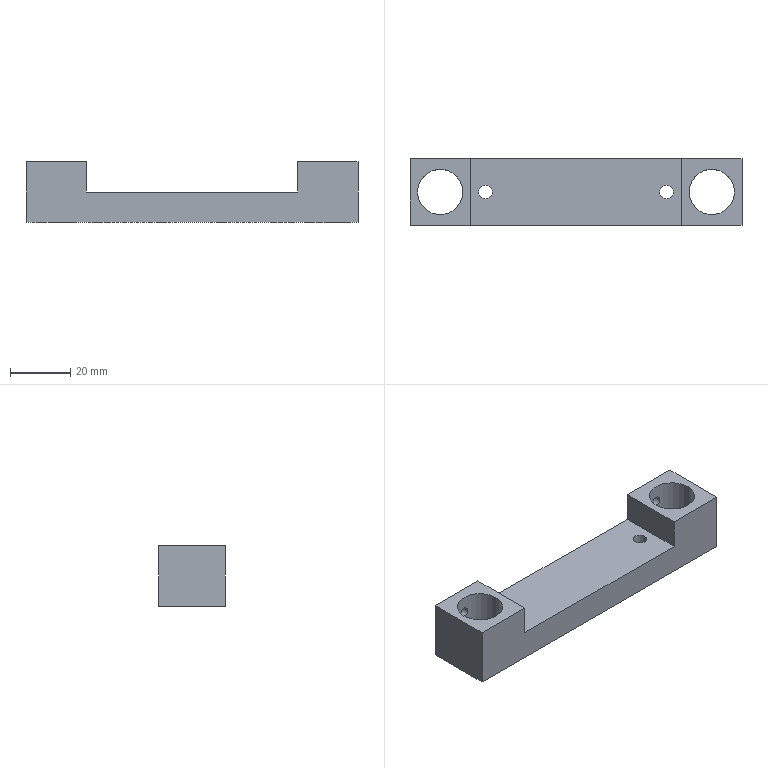Part | STEP file | XL-005 | 1 solid | 38 faces | box 110 x 22 x 20 mm | volume 25117 mm3 | cylinder 24 | plane 14 | commonest cylinder face diameters 3.3 x8 2.5 x4 4.5 x4 8 x4 15 x4
STEP:
#1=CARTESIAN_POINT('',(89.,11.,4.6));
#2=VERTEX_POINT('',#1);
#3=CARTESIAN_POINT('',(81.,11.,4.6));
#4=VERTEX_POINT('',#3);
#5=CARTESIAN_POINT('',(85.,11.,4.6));
#6=DIRECTION('',(0.,0.,-1.));
#7=DIRECTION('',(-1.,0.,0.));
#8=AXIS2_PLACEMENT_3D('',#5,#6,#7);
#9=CIRCLE('',#8,4.);
#10=EDGE_CURVE('',#2,#4,#9,.T.);
#11=ORIENTED_EDGE('',*,*,#10,.F.);
#12=CARTESIAN_POINT('',(89.,11.,0.));
#13=VERTEX_POINT('',#12);
#14=CARTESIAN_POINT('',(89.,11.,0.));
#15=DIRECTION('',(0.,0.,-1.));
#16=VECTOR('',#15,1000.);
#17=LINE('',#14,#16);
#18=EDGE_CURVE('',#2,#13,#17,.T.);
#19=ORIENTED_EDGE('',*,*,#18,.T.);
#20=CARTESIAN_POINT('',(81.,11.,0.));
#21=VERTEX_POINT('',#20);
#22=CARTESIAN_POINT('',(85.,11.,0.));
#23=DIRECTION('',(0.,0.,-1.));
#24=DIRECTION('',(-1.,0.,0.));
#25=AXIS2_PLACEMENT_3D('',#22,#23,#24);
#26=CIRCLE('',#25,4.);
#27=EDGE_CURVE('',#13,#21,#26,.T.);
#28=ORIENTED_EDGE('',*,*,#27,.T.);
#29=CARTESIAN_POINT('',(81.,11.,0.));
#30=DIRECTION('',(0.,0.,-1.));
#31=VECTOR('',#30,1000.);
#32=LINE('',#29,#31);
#33=EDGE_CURVE('',#4,#21,#32,.T.);
#34=ORIENTED_EDGE('',*,*,#33,.F.);
#35=EDGE_LOOP('',(#11,#19,#28,#34));
#36=FACE_OUTER_BOUND('',#35,.T.);
#37=CARTESIAN_POINT('',(85.,11.,0.));
#38=DIRECTION('',(0.,0.,-1.));
#39=DIRECTION('',(-1.,0.,0.));
#40=AXIS2_PLACEMENT_3D('',#37,#38,#39);
#41=CYLINDRICAL_SURFACE('',#40,4.);
#42=ADVANCED_FACE('',(#36),#41,.F.);
#43=CARTESIAN_POINT('',(82.75,11.,10.));
#44=VERTEX_POINT('',#43);
#45=CARTESIAN_POINT('',(87.25,11.,10.));
#46=VERTEX_POINT('',#45);
#47=CARTESIAN_POINT('',(85.,11.,10.));
#48=DIRECTION('',(0.,0.,1.));
#49=DIRECTION('',(1.,0.,0.));
#50=AXIS2_PLACEMENT_3D('',#47,#48,#49);
#51=CIRCLE('',#50,2.25);
#52=EDGE_CURVE('',#44,#46,#51,.T.);
#53=ORIENTED_EDGE('',*,*,#52,.T.);
#54=CARTESIAN_POINT('',(87.25,11.,4.6));
#55=VERTEX_POINT('',#54);
#56=CARTESIAN_POINT('',(87.25,11.,0.));
#57=DIRECTION('',(0.,0.,-1.));
#58=VECTOR('',#57,1000.);
#59=LINE('',#56,#58);
#60=EDGE_CURVE('',#46,#55,#59,.T.);
#61=ORIENTED_EDGE('',*,*,#60,.T.);
#62=CARTESIAN_POINT('',(82.75,11.,4.6));
#63=VERTEX_POINT('',#62);
#64=CARTESIAN_POINT('',(85.,11.,4.6));
#65=DIRECTION('',(0.,0.,-1.));
#66=DIRECTION('',(-1.,0.,0.));
#67=AXIS2_PLACEMENT_3D('',#64,#65,#66);
#68=CIRCLE('',#67,2.25);
#69=EDGE_CURVE('',#55,#63,#68,.T.);
#70=ORIENTED_EDGE('',*,*,#69,.T.);
#71=CARTESIAN_POINT('',(82.75,11.,0.));
#72=DIRECTION('',(0.,0.,-1.));
#73=VECTOR('',#72,1000.);
#74=LINE('',#71,#73);
#75=EDGE_CURVE('',#44,#63,#74,.T.);
#76=ORIENTED_EDGE('',*,*,#75,.F.);
#77=EDGE_LOOP('',(#53,#61,#70,#76));
#78=FACE_OUTER_BOUND('',#77,.T.);
#79=CARTESIAN_POINT('',(85.,11.,0.));
#80=DIRECTION('',(0.,0.,-1.));
#81=DIRECTION('',(-1.,0.,0.));
#82=AXIS2_PLACEMENT_3D('',#79,#80,#81);
#83=CYLINDRICAL_SURFACE('',#82,2.25);
#84=ADVANCED_FACE('',(#78),#83,.F.);
#85=CARTESIAN_POINT('',(29.,11.,4.6));
#86=VERTEX_POINT('',#85);
#87=CARTESIAN_POINT('',(21.,11.,4.6));
#88=VERTEX_POINT('',#87);
#89=CARTESIAN_POINT('',(25.,11.,4.6));
#90=DIRECTION('',(0.,0.,-1.));
#91=DIRECTION('',(-1.,0.,0.));
#92=AXIS2_PLACEMENT_3D('',#89,#90,#91);
#93=CIRCLE('',#92,4.);
#94=EDGE_CURVE('',#86,#88,#93,.T.);
#95=ORIENTED_EDGE('',*,*,#94,.F.);
#96=CARTESIAN_POINT('',(29.,11.,0.));
#97=VERTEX_POINT('',#96);
#98=CARTESIAN_POINT('',(29.,11.,0.));
#99=DIRECTION('',(0.,0.,-1.));
#100=VECTOR('',#99,1000.);
#101=LINE('',#98,#100);
#102=EDGE_CURVE('',#86,#97,#101,.T.);
#103=ORIENTED_EDGE('',*,*,#102,.T.);
#104=CARTESIAN_POINT('',(21.,11.,0.));
#105=VERTEX_POINT('',#104);
#106=CARTESIAN_POINT('',(25.,11.,0.));
#107=DIRECTION('',(0.,0.,-1.));
#108=DIRECTION('',(-1.,0.,0.));
#109=AXIS2_PLACEMENT_3D('',#106,#107,#108);
#110=CIRCLE('',#109,4.);
#111=EDGE_CURVE('',#97,#105,#110,.T.);
#112=ORIENTED_EDGE('',*,*,#111,.T.);
#113=CARTESIAN_POINT('',(21.,11.,0.));
#114=DIRECTION('',(0.,0.,-1.));
#115=VECTOR('',#114,1000.);
#116=LINE('',#113,#115);
#117=EDGE_CURVE('',#88,#105,#116,.T.);
#118=ORIENTED_EDGE('',*,*,#117,.F.);
#119=EDGE_LOOP('',(#95,#103,#112,#118));
#120=FACE_OUTER_BOUND('',#119,.T.);
#121=CARTESIAN_POINT('',(25.,11.,0.));
#122=DIRECTION('',(0.,0.,-1.));
#123=DIRECTION('',(-1.,0.,0.));
#124=AXIS2_PLACEMENT_3D('',#121,#122,#123);
#125=CYLINDRICAL_SURFACE('',#124,4.);
#126=ADVANCED_FACE('',(#120),#125,.F.);
#127=CARTESIAN_POINT('',(22.75,11.,10.));
#128=VERTEX_POINT('',#127);
#129=CARTESIAN_POINT('',(27.25,11.,10.));
#130=VERTEX_POINT('',#129);
#131=CARTESIAN_POINT('',(25.,11.,10.));
#132=DIRECTION('',(0.,0.,1.));
#133=DIRECTION('',(1.,0.,0.));
#134=AXIS2_PLACEMENT_3D('',#131,#132,#133);
#135=CIRCLE('',#134,2.25);
#136=EDGE_CURVE('',#128,#130,#135,.T.);
#137=ORIENTED_EDGE('',*,*,#136,.T.);
#138=CARTESIAN_POINT('',(27.25,11.,4.6));
#139=VERTEX_POINT('',#138);
#140=CARTESIAN_POINT('',(27.25,11.,0.));
#141=DIRECTION('',(0.,0.,-1.));
#142=VECTOR('',#141,1000.);
#143=LINE('',#140,#142);
#144=EDGE_CURVE('',#130,#139,#143,.T.);
#145=ORIENTED_EDGE('',*,*,#144,.T.);
#146=CARTESIAN_POINT('',(22.75,11.,4.6));
#147=VERTEX_POINT('',#146);
#148=CARTESIAN_POINT('',(25.,11.,4.6));
#149=DIRECTION('',(0.,0.,-1.));
#150=DIRECTION('',(-1.,0.,0.));
#151=AXIS2_PLACEMENT_3D('',#148,#149,#150);
#152=CIRCLE('',#151,2.25);
#153=EDGE_CURVE('',#139,#147,#152,.T.);
#154=ORIENTED_EDGE('',*,*,#153,.T.);
#155=CARTESIAN_POINT('',(22.75,11.,0.));
#156=DIRECTION('',(0.,0.,-1.));
#157=VECTOR('',#156,1000.);
#158=LINE('',#155,#157);
#159=EDGE_CURVE('',#128,#147,#158,.T.);
#160=ORIENTED_EDGE('',*,*,#159,.F.);
#161=EDGE_LOOP('',(#137,#145,#154,#160));
#162=FACE_OUTER_BOUND('',#161,.T.);
#163=CARTESIAN_POINT('',(25.,11.,0.));
#164=DIRECTION('',(0.,0.,-1.));
#165=DIRECTION('',(-1.,0.,0.));
#166=AXIS2_PLACEMENT_3D('',#163,#164,#165);
#167=CYLINDRICAL_SURFACE('',#166,2.25);
#168=ADVANCED_FACE('',(#162),#167,.F.);
#169=CARTESIAN_POINT('',(66.25,11.,6.));
#170=VERTEX_POINT('',#169);
#171=CARTESIAN_POINT('',(63.75,11.,6.));
#172=VERTEX_POINT('',#171);
#173=CARTESIAN_POINT('',(65.,11.,6.));
#174=DIRECTION('',(0.,0.,-1.));
#175=DIRECTION('',(-1.,0.,0.));
#176=AXIS2_PLACEMENT_3D('',#173,#174,#175);
#177=CIRCLE('',#176,1.25);
#178=EDGE_CURVE('',#170,#172,#177,.T.);
#179=ORIENTED_EDGE('',*,*,#178,.F.);
#180=CARTESIAN_POINT('',(66.25,11.,0.));
#181=VERTEX_POINT('',#180);
#182=CARTESIAN_POINT('',(66.25,11.,6.));
#183=DIRECTION('',(0.,0.,-1.));
#184=VECTOR('',#183,1000.);
#185=LINE('',#182,#184);
#186=EDGE_CURVE('',#170,#181,#185,.T.);
#187=ORIENTED_EDGE('',*,*,#186,.T.);
#188=CARTESIAN_POINT('',(63.75,11.,0.));
#189=VERTEX_POINT('',#188);
#190=CARTESIAN_POINT('',(65.,11.,0.));
#191=DIRECTION('',(0.,0.,-1.));
#192=DIRECTION('',(-1.,0.,0.));
#193=AXIS2_PLACEMENT_3D('',#190,#191,#192);
#194=CIRCLE('',#193,1.25);
#195=EDGE_CURVE('',#181,#189,#194,.T.);
#196=ORIENTED_EDGE('',*,*,#195,.T.);
#197=CARTESIAN_POINT('',(63.75,11.,6.));
#198=DIRECTION('',(0.,0.,-1.));
#199=VECTOR('',#198,1000.);
#200=LINE('',#197,#199);
#201=EDGE_CURVE('',#172,#189,#200,.T.);
#202=ORIENTED_EDGE('',*,*,#201,.F.);
#203=EDGE_LOOP('',(#179,#187,#196,#202));
#204=FACE_OUTER_BOUND('',#203,.T.);
#205=CARTESIAN_POINT('',(65.,11.,6.));
#206=DIRECTION('',(0.,0.,-1.));
#207=DIRECTION('',(-1.,0.,0.));
#208=AXIS2_PLACEMENT_3D('',#205,#206,#207);
#209=CYLINDRICAL_SURFACE('',#208,1.25);
#210=ADVANCED_FACE('',(#204),#209,.F.);
#211=CARTESIAN_POINT('',(46.25,11.,6.));
#212=VERTEX_POINT('',#211);
#213=CARTESIAN_POINT('',(43.75,11.,6.));
#214=VERTEX_POINT('',#213);
#215=CARTESIAN_POINT('',(45.,11.,6.));
#216=DIRECTION('',(0.,0.,-1.));
#217=DIRECTION('',(-1.,0.,0.));
#218=AXIS2_PLACEMENT_3D('',#215,#216,#217);
#219=CIRCLE('',#218,1.25);
#220=EDGE_CURVE('',#212,#214,#219,.T.);
#221=ORIENTED_EDGE('',*,*,#220,.F.);
#222=CARTESIAN_POINT('',(46.25,11.,0.));
#223=VERTEX_POINT('',#222);
#224=CARTESIAN_POINT('',(46.25,11.,6.));
#225=DIRECTION('',(0.,0.,-1.));
#226=VECTOR('',#225,1000.);
#227=LINE('',#224,#226);
#228=EDGE_CURVE('',#212,#223,#227,.T.);
#229=ORIENTED_EDGE('',*,*,#228,.T.);
#230=CARTESIAN_POINT('',(43.75,11.,0.));
#231=VERTEX_POINT('',#230);
#232=CARTESIAN_POINT('',(45.,11.,0.));
#233=DIRECTION('',(0.,0.,-1.));
#234=DIRECTION('',(-1.,0.,0.));
#235=AXIS2_PLACEMENT_3D('',#232,#233,#234);
#236=CIRCLE('',#235,1.25);
#237=EDGE_CURVE('',#223,#231,#236,.T.);
#238=ORIENTED_EDGE('',*,*,#237,.T.);
#239=CARTESIAN_POINT('',(43.75,11.,6.));
#240=DIRECTION('',(0.,0.,-1.));
#241=VECTOR('',#240,1000.);
#242=LINE('',#239,#241);
#243=EDGE_CURVE('',#214,#231,#242,.T.);
#244=ORIENTED_EDGE('',*,*,#243,.F.);
#245=EDGE_LOOP('',(#221,#229,#238,#244));
#246=FACE_OUTER_BOUND('',#245,.T.);
#247=CARTESIAN_POINT('',(45.,11.,6.));
#248=DIRECTION('',(0.,0.,-1.));
#249=DIRECTION('',(-1.,0.,0.));
#250=AXIS2_PLACEMENT_3D('',#247,#248,#249);
#251=CYLINDRICAL_SURFACE('',#250,1.25);
#252=ADVANCED_FACE('',(#246),#251,.F.);
#253=CARTESIAN_POINT('',(100.,18.5,7.65));
#254=VERTEX_POINT('',#253);
#255=CARTESIAN_POINT('',(100.,18.5,4.35));
#256=VERTEX_POINT('',#255);
#257=CARTESIAN_POINT('',(100.,18.5,7.65));
#258=CARTESIAN_POINT('',(99.891,18.5,7.65));
#259=CARTESIAN_POINT('',(99.783,18.498,7.639));
#260=CARTESIAN_POINT('',(99.572,18.489,7.597));
#261=CARTESIAN_POINT('',(99.467,18.482,7.565));
#262=CARTESIAN_POINT('',(99.267,18.465,7.482));
#263=CARTESIAN_POINT('',(99.172,18.455,7.432));
#264=CARTESIAN_POINT('',(98.993,18.433,7.312));
#265=CARTESIAN_POINT('',(98.909,18.421,7.242));
#266=CARTESIAN_POINT('',(98.681,18.385,7.015));
#267=CARTESIAN_POINT('',(98.558,18.361,6.831));
#268=CARTESIAN_POINT('',(98.394,18.326,6.434));
#269=CARTESIAN_POINT('',(98.35,18.316,6.217));
#270=CARTESIAN_POINT('',(98.35,18.316,5.893));
#271=CARTESIAN_POINT('',(98.361,18.319,5.783));
#272=CARTESIAN_POINT('',(98.403,18.328,5.571));
#273=CARTESIAN_POINT('',(98.434,18.335,5.468));
#274=CARTESIAN_POINT('',(98.559,18.361,5.168));
#275=CARTESIAN_POINT('',(98.68,18.385,4.986));
#276=CARTESIAN_POINT('',(98.91,18.421,4.757));
#277=CARTESIAN_POINT('',(98.993,18.433,4.689));
#278=CARTESIAN_POINT('',(99.171,18.455,4.569));
#279=CARTESIAN_POINT('',(99.268,18.465,4.517));
#280=CARTESIAN_POINT('',(99.467,18.482,4.435));
#281=CARTESIAN_POINT('',(99.57,18.488,4.403));
#282=CARTESIAN_POINT('',(99.783,18.498,4.361));
#283=CARTESIAN_POINT('',(99.892,18.5,4.35));
#284=CARTESIAN_POINT('',(100.,18.5,4.35));
#285=B_SPLINE_CURVE_WITH_KNOTS('',3,(#257,#258,#259,#260,#261,#262,#263,#264,#265,#266,#267,#268,#269,#270,#271,#272,#273,#274,#275,#276,#277,#278,#279,#280,#281,#282,#283,#284),.UNSPECIFIED.,.F.,.F.,(4,2,2,2,2,2,2,2,2,2,2,2,2,4),(0.,0.0003234,0.0006468,0.0009702,0.001294,0.00194,0.002587,0.002911,0.003234,0.003881,0.004204,0.004528,0.004851,0.005175),.UNSPECIFIED.);
#286=EDGE_CURVE('',#254,#256,#285,.T.);
#287=ORIENTED_EDGE('',*,*,#286,.T.);
#288=CARTESIAN_POINT('',(100.,22.,4.35));
#289=VERTEX_POINT('',#288);
#290=CARTESIAN_POINT('',(100.,-0.001,4.35));
#291=DIRECTION('',(0.,1.,0.));
#292=VECTOR('',#291,1000.);
#293=LINE('',#290,#292);
#294=EDGE_CURVE('',#256,#289,#293,.T.);
#295=ORIENTED_EDGE('',*,*,#294,.T.);
#296=CARTESIAN_POINT('',(100.,22.,7.65));
#297=VERTEX_POINT('',#296);
#298=CARTESIAN_POINT('',(100.,22.,6.));
#299=DIRECTION('',(0.,1.,0.));
#300=DIRECTION('',(0.,0.,-1.));
#301=AXIS2_PLACEMENT_3D('',#298,#299,#300);
#302=CIRCLE('',#301,1.65);
#303=EDGE_CURVE('',#289,#297,#302,.T.);
#304=ORIENTED_EDGE('',*,*,#303,.T.);
#305=CARTESIAN_POINT('',(100.,-0.001,7.65));
#306=DIRECTION('',(0.,1.,0.));
#307=VECTOR('',#306,1000.);
#308=LINE('',#305,#307);
#309=EDGE_CURVE('',#254,#297,#308,.T.);
#310=ORIENTED_EDGE('',*,*,#309,.F.);
#311=EDGE_LOOP('',(#287,#295,#304,#310));
#312=FACE_OUTER_BOUND('',#311,.T.);
#313=CARTESIAN_POINT('',(100.,-0.001,6.));
#314=DIRECTION('',(0.,1.,0.));
#315=DIRECTION('',(0.,0.,1.));
#316=AXIS2_PLACEMENT_3D('',#313,#314,#315);
#317=CYLINDRICAL_SURFACE('',#316,1.65);
#318=ADVANCED_FACE('',(#312),#317,.F.);
#319=CARTESIAN_POINT('',(100.,18.5,15.65));
#320=VERTEX_POINT('',#319);
#321=CARTESIAN_POINT('',(100.,18.5,12.35));
#322=VERTEX_POINT('',#321);
#323=CARTESIAN_POINT('',(100.,18.5,15.65));
#324=CARTESIAN_POINT('',(99.891,18.5,15.65));
#325=CARTESIAN_POINT('',(99.783,18.498,15.639));
#326=CARTESIAN_POINT('',(99.572,18.489,15.597));
#327=CARTESIAN_POINT('',(99.467,18.482,15.565));
#328=CARTESIAN_POINT('',(99.267,18.465,15.482));
#329=CARTESIAN_POINT('',(99.172,18.455,15.432));
#330=CARTESIAN_POINT('',(98.993,18.433,15.312));
#331=CARTESIAN_POINT('',(98.909,18.421,15.242));
#332=CARTESIAN_POINT('',(98.681,18.385,15.015));
#333=CARTESIAN_POINT('',(98.558,18.361,14.831));
#334=CARTESIAN_POINT('',(98.394,18.326,14.434));
#335=CARTESIAN_POINT('',(98.35,18.316,14.217));
#336=CARTESIAN_POINT('',(98.35,18.316,13.893));
#337=CARTESIAN_POINT('',(98.361,18.319,13.783));
#338=CARTESIAN_POINT('',(98.403,18.328,13.571));
#339=CARTESIAN_POINT('',(98.434,18.335,13.468));
#340=CARTESIAN_POINT('',(98.559,18.361,13.168));
#341=CARTESIAN_POINT('',(98.68,18.385,12.986));
#342=CARTESIAN_POINT('',(98.91,18.421,12.757));
#343=CARTESIAN_POINT('',(98.993,18.433,12.689));
#344=CARTESIAN_POINT('',(99.171,18.455,12.569));
#345=CARTESIAN_POINT('',(99.268,18.465,12.517));
#346=CARTESIAN_POINT('',(99.467,18.482,12.435));
#347=CARTESIAN_POINT('',(99.57,18.488,12.403));
#348=CARTESIAN_POINT('',(99.783,18.498,12.361));
#349=CARTESIAN_POINT('',(99.892,18.5,12.35));
#350=CARTESIAN_POINT('',(100.,18.5,12.35));
#351=B_SPLINE_CURVE_WITH_KNOTS('',3,(#323,#324,#325,#326,#327,#328,#329,#330,#331,#332,#333,#334,#335,#336,#337,#338,#339,#340,#341,#342,#343,#344,#345,#346,#347,#348,#349,#350),.UNSPECIFIED.,.F.,.F.,(4,2,2,2,2,2,2,2,2,2,2,2,2,4),(0.,0.0003234,0.0006468,0.0009702,0.001294,0.00194,0.002587,0.002911,0.003234,0.003881,0.004204,0.004528,0.004851,0.005175),.UNSPECIFIED.);
#352=EDGE_CURVE('',#320,#322,#351,.T.);
#353=ORIENTED_EDGE('',*,*,#352,.T.);
#354=CARTESIAN_POINT('',(100.,22.,12.35));
#355=VERTEX_POINT('',#354);
#356=CARTESIAN_POINT('',(100.,-0.001,12.35));
#357=DIRECTION('',(0.,1.,0.));
#358=VECTOR('',#357,1000.);
#359=LINE('',#356,#358);
#360=EDGE_CURVE('',#322,#355,#359,.T.);
#361=ORIENTED_EDGE('',*,*,#360,.T.);
#362=CARTESIAN_POINT('',(100.,22.,15.65));
#363=VERTEX_POINT('',#362);
#364=CARTESIAN_POINT('',(100.,22.,14.));
#365=DIRECTION('',(0.,1.,0.));
#366=DIRECTION('',(0.,0.,-1.));
#367=AXIS2_PLACEMENT_3D('',#364,#365,#366);
#368=CIRCLE('',#367,1.65);
#369=EDGE_CURVE('',#355,#363,#368,.T.);
#370=ORIENTED_EDGE('',*,*,#369,.T.);
#371=CARTESIAN_POINT('',(100.,-0.001,15.65));
#372=DIRECTION('',(0.,1.,0.));
#373=VECTOR('',#372,1000.);
#374=LINE('',#371,#373);
#375=EDGE_CURVE('',#320,#363,#374,.T.);
#376=ORIENTED_EDGE('',*,*,#375,.F.);
#377=EDGE_LOOP('',(#353,#361,#370,#376));
#378=FACE_OUTER_BOUND('',#377,.T.);
#379=CARTESIAN_POINT('',(100.,-0.001,14.));
#380=DIRECTION('',(0.,1.,0.));
#381=DIRECTION('',(0.,0.,1.));
#382=AXIS2_PLACEMENT_3D('',#379,#380,#381);
#383=CYLINDRICAL_SURFACE('',#382,1.65);
#384=ADVANCED_FACE('',(#378),#383,.F.);
#385=CARTESIAN_POINT('',(10.,18.5,15.65));
#386=VERTEX_POINT('',#385);
#387=CARTESIAN_POINT('',(10.,18.5,12.35));
#388=VERTEX_POINT('',#387);
#389=CARTESIAN_POINT('',(10.,18.5,15.65));
#390=CARTESIAN_POINT('',(9.891,18.5,15.65));
#391=CARTESIAN_POINT('',(9.783,18.498,15.639));
#392=CARTESIAN_POINT('',(9.572,18.489,15.597));
#393=CARTESIAN_POINT('',(9.467,18.482,15.565));
#394=CARTESIAN_POINT('',(9.267,18.465,15.482));
#395=CARTESIAN_POINT('',(9.172,18.455,15.432));
#396=CARTESIAN_POINT('',(8.993,18.433,15.312));
#397=CARTESIAN_POINT('',(8.909,18.421,15.242));
#398=CARTESIAN_POINT('',(8.681,18.385,15.015));
#399=CARTESIAN_POINT('',(8.558,18.361,14.831));
#400=CARTESIAN_POINT('',(8.394,18.326,14.434));
#401=CARTESIAN_POINT('',(8.35,18.316,14.217));
#402=CARTESIAN_POINT('',(8.35,18.316,13.893));
#403=CARTESIAN_POINT('',(8.361,18.319,13.783));
#404=CARTESIAN_POINT('',(8.403,18.328,13.571));
#405=CARTESIAN_POINT('',(8.434,18.335,13.468));
#406=CARTESIAN_POINT('',(8.559,18.361,13.168));
#407=CARTESIAN_POINT('',(8.68,18.385,12.986));
#408=CARTESIAN_POINT('',(8.91,18.421,12.757));
#409=CARTESIAN_POINT('',(8.993,18.433,12.689));
#410=CARTESIAN_POINT('',(9.171,18.455,12.569));
#411=CARTESIAN_POINT('',(9.268,18.465,12.517));
#412=CARTESIAN_POINT('',(9.467,18.482,12.435));
#413=CARTESIAN_POINT('',(9.57,18.488,12.403));
#414=CARTESIAN_POINT('',(9.783,18.498,12.361));
#415=CARTESIAN_POINT('',(9.892,18.5,12.35));
#416=CARTESIAN_POINT('',(10.,18.5,12.35));
#417=B_SPLINE_CURVE_WITH_KNOTS('',3,(#389,#390,#391,#392,#393,#394,#395,#396,#397,#398,#399,#400,#401,#402,#403,#404,#405,#406,#407,#408,#409,#410,#411,#412,#413,#414,#415,#416),.UNSPECIFIED.,.F.,.F.,(4,2,2,2,2,2,2,2,2,2,2,2,2,4),(0.,0.0003234,0.0006468,0.0009702,0.001294,0.00194,0.002587,0.002911,0.003234,0.003881,0.004204,0.004528,0.004851,0.005175),.UNSPECIFIED.);
#418=EDGE_CURVE('',#386,#388,#417,.T.);
#419=ORIENTED_EDGE('',*,*,#418,.T.);
#420=CARTESIAN_POINT('',(10.,22.,12.35));
#421=VERTEX_POINT('',#420);
#422=CARTESIAN_POINT('',(10.,-0.001,12.35));
#423=DIRECTION('',(0.,1.,0.));
#424=VECTOR('',#423,1000.);
#425=LINE('',#422,#424);
#426=EDGE_CURVE('',#388,#421,#425,.T.);
#427=ORIENTED_EDGE('',*,*,#426,.T.);
#428=CARTESIAN_POINT('',(10.,22.,15.65));
#429=VERTEX_POINT('',#428);
#430=CARTESIAN_POINT('',(10.,22.,14.));
#431=DIRECTION('',(0.,1.,0.));
#432=DIRECTION('',(0.,0.,1.));
#433=AXIS2_PLACEMENT_3D('',#430,#431,#432);
#434=CIRCLE('',#433,1.65);
#435=EDGE_CURVE('',#421,#429,#434,.T.);
#436=ORIENTED_EDGE('',*,*,#435,.T.);
#437=CARTESIAN_POINT('',(10.,-0.001,15.65));
#438=DIRECTION('',(0.,1.,0.));
#439=VECTOR('',#438,1000.);
#440=LINE('',#437,#439);
#441=EDGE_CURVE('',#386,#429,#440,.T.);
#442=ORIENTED_EDGE('',*,*,#441,.F.);
#443=EDGE_LOOP('',(#419,#427,#436,#442));
#444=FACE_OUTER_BOUND('',#443,.T.);
#445=CARTESIAN_POINT('',(10.,-0.001,14.));
#446=DIRECTION('',(0.,1.,0.));
#447=DIRECTION('',(0.,0.,1.));
#448=AXIS2_PLACEMENT_3D('',#445,#446,#447);
#449=CYLINDRICAL_SURFACE('',#448,1.65);
#450=ADVANCED_FACE('',(#444),#449,.F.);
#451=CARTESIAN_POINT('',(10.,18.5,7.65));
#452=VERTEX_POINT('',#451);
#453=CARTESIAN_POINT('',(10.,18.5,4.35));
#454=VERTEX_POINT('',#453);
#455=CARTESIAN_POINT('',(10.,18.5,7.65));
#456=CARTESIAN_POINT('',(9.891,18.5,7.65));
#457=CARTESIAN_POINT('',(9.783,18.498,7.639));
#458=CARTESIAN_POINT('',(9.572,18.489,7.597));
#459=CARTESIAN_POINT('',(9.467,18.482,7.565));
#460=CARTESIAN_POINT('',(9.267,18.465,7.482));
#461=CARTESIAN_POINT('',(9.172,18.455,7.432));
#462=CARTESIAN_POINT('',(8.993,18.433,7.312));
#463=CARTESIAN_POINT('',(8.909,18.421,7.242));
#464=CARTESIAN_POINT('',(8.681,18.385,7.015));
#465=CARTESIAN_POINT('',(8.558,18.361,6.831));
#466=CARTESIAN_POINT('',(8.394,18.326,6.434));
#467=CARTESIAN_POINT('',(8.35,18.316,6.217));
#468=CARTESIAN_POINT('',(8.35,18.316,5.893));
#469=CARTESIAN_POINT('',(8.361,18.319,5.783));
#470=CARTESIAN_POINT('',(8.403,18.328,5.571));
#471=CARTESIAN_POINT('',(8.434,18.335,5.468));
#472=CARTESIAN_POINT('',(8.559,18.361,5.168));
#473=CARTESIAN_POINT('',(8.68,18.385,4.986));
#474=CARTESIAN_POINT('',(8.91,18.421,4.757));
#475=CARTESIAN_POINT('',(8.993,18.433,4.689));
#476=CARTESIAN_POINT('',(9.171,18.455,4.569));
#477=CARTESIAN_POINT('',(9.268,18.465,4.517));
#478=CARTESIAN_POINT('',(9.467,18.482,4.435));
#479=CARTESIAN_POINT('',(9.57,18.488,4.403));
#480=CARTESIAN_POINT('',(9.783,18.498,4.361));
#481=CARTESIAN_POINT('',(9.892,18.5,4.35));
#482=CARTESIAN_POINT('',(10.,18.5,4.35));
#483=B_SPLINE_CURVE_WITH_KNOTS('',3,(#455,#456,#457,#458,#459,#460,#461,#462,#463,#464,#465,#466,#467,#468,#469,#470,#471,#472,#473,#474,#475,#476,#477,#478,#479,#480,#481,#482),.UNSPECIFIED.,.F.,.F.,(4,2,2,2,2,2,2,2,2,2,2,2,2,4),(0.,0.0003234,0.0006468,0.0009702,0.001294,0.00194,0.002587,0.002911,0.003234,0.003881,0.004204,0.004528,0.004851,0.005175),.UNSPECIFIED.);
#484=EDGE_CURVE('',#452,#454,#483,.T.);
#485=ORIENTED_EDGE('',*,*,#484,.T.);
#486=CARTESIAN_POINT('',(10.,22.,4.35));
#487=VERTEX_POINT('',#486);
#488=CARTESIAN_POINT('',(10.,-0.001,4.35));
#489=DIRECTION('',(0.,1.,0.));
#490=VECTOR('',#489,1000.);
#491=LINE('',#488,#490);
#492=EDGE_CURVE('',#454,#487,#491,.T.);
#493=ORIENTED_EDGE('',*,*,#492,.T.);
#494=CARTESIAN_POINT('',(10.,22.,7.65));
#495=VERTEX_POINT('',#494);
#496=CARTESIAN_POINT('',(10.,22.,6.));
#497=DIRECTION('',(0.,1.,0.));
#498=DIRECTION('',(0.,0.,1.));
#499=AXIS2_PLACEMENT_3D('',#496,#497,#498);
#500=CIRCLE('',#499,1.65);
#501=EDGE_CURVE('',#487,#495,#500,.T.);
#502=ORIENTED_EDGE('',*,*,#501,.T.);
#503=CARTESIAN_POINT('',(10.,-0.001,7.65));
#504=DIRECTION('',(0.,1.,0.));
#505=VECTOR('',#504,1000.);
#506=LINE('',#503,#505);
#507=EDGE_CURVE('',#452,#495,#506,.T.);
#508=ORIENTED_EDGE('',*,*,#507,.F.);
#509=EDGE_LOOP('',(#485,#493,#502,#508));
#510=FACE_OUTER_BOUND('',#509,.T.);
#511=CARTESIAN_POINT('',(10.,-0.001,6.));
#512=DIRECTION('',(0.,1.,0.));
#513=DIRECTION('',(0.,0.,1.));
#514=AXIS2_PLACEMENT_3D('',#511,#512,#513);
#515=CYLINDRICAL_SURFACE('',#514,1.65);
#516=ADVANCED_FACE('',(#510),#515,.F.);
#517=CARTESIAN_POINT('',(2.5,11.,0.));
#518=VERTEX_POINT('',#517);
#519=CARTESIAN_POINT('',(17.5,11.,0.));
#520=VERTEX_POINT('',#519);
#521=CARTESIAN_POINT('',(10.,11.,0.));
#522=DIRECTION('',(0.,0.,1.));
#523=DIRECTION('',(1.,0.,0.));
#524=AXIS2_PLACEMENT_3D('',#521,#522,#523);
#525=CIRCLE('',#524,7.5);
#526=EDGE_CURVE('',#518,#520,#525,.T.);
#527=ORIENTED_EDGE('',*,*,#526,.F.);
#528=CARTESIAN_POINT('',(2.5,11.,20.));
#529=VERTEX_POINT('',#528);
#530=CARTESIAN_POINT('',(2.5,11.,0.));
#531=DIRECTION('',(0.,0.,1.));
#532=VECTOR('',#531,1000.);
#533=LINE('',#530,#532);
#534=EDGE_CURVE('',#518,#529,#533,.T.);
#535=ORIENTED_EDGE('',*,*,#534,.T.);
#536=CARTESIAN_POINT('',(17.5,11.,20.));
#537=VERTEX_POINT('',#536);
#538=CARTESIAN_POINT('',(10.,11.,20.));
#539=DIRECTION('',(0.,0.,1.));
#540=DIRECTION('',(1.,0.,0.));
#541=AXIS2_PLACEMENT_3D('',#538,#539,#540);
#542=CIRCLE('',#541,7.5);
#543=EDGE_CURVE('',#529,#537,#542,.T.);
#544=ORIENTED_EDGE('',*,*,#543,.T.);
#545=CARTESIAN_POINT('',(17.5,11.,0.));
#546=DIRECTION('',(0.,0.,1.));
#547=VECTOR('',#546,1000.);
#548=LINE('',#545,#547);
#549=EDGE_CURVE('',#520,#537,#548,.T.);
#550=ORIENTED_EDGE('',*,*,#549,.F.);
#551=EDGE_LOOP('',(#527,#535,#544,#550));
#552=FACE_OUTER_BOUND('',#551,.T.);
#553=CARTESIAN_POINT('',(10.,11.,0.));
#554=DIRECTION('',(0.,0.,1.));
#555=DIRECTION('',(1.,0.,0.));
#556=AXIS2_PLACEMENT_3D('',#553,#554,#555);
#557=CYLINDRICAL_SURFACE('',#556,7.5);
#558=ADVANCED_FACE('',(#552),#557,.F.);
#559=CARTESIAN_POINT('',(92.5,11.,0.));
#560=VERTEX_POINT('',#559);
#561=CARTESIAN_POINT('',(107.5,11.,0.));
#562=VERTEX_POINT('',#561);
#563=CARTESIAN_POINT('',(100.,11.,0.));
#564=DIRECTION('',(0.,0.,1.));
#565=DIRECTION('',(-1.,0.,0.));
#566=AXIS2_PLACEMENT_3D('',#563,#564,#565);
#567=CIRCLE('',#566,7.5);
#568=EDGE_CURVE('',#560,#562,#567,.T.);
#569=ORIENTED_EDGE('',*,*,#568,.F.);
#570=CARTESIAN_POINT('',(92.5,11.,20.));
#571=VERTEX_POINT('',#570);
#572=CARTESIAN_POINT('',(92.5,11.,0.));
#573=DIRECTION('',(0.,0.,1.));
#574=VECTOR('',#573,1000.);
#575=LINE('',#572,#574);
#576=EDGE_CURVE('',#560,#571,#575,.T.);
#577=ORIENTED_EDGE('',*,*,#576,.T.);
#578=CARTESIAN_POINT('',(107.5,11.,20.));
#579=VERTEX_POINT('',#578);
#580=CARTESIAN_POINT('',(100.,11.,20.));
#581=DIRECTION('',(0.,0.,1.));
#582=DIRECTION('',(-1.,0.,0.));
#583=AXIS2_PLACEMENT_3D('',#580,#581,#582);
#584=CIRCLE('',#583,7.5);
#585=EDGE_CURVE('',#571,#579,#584,.T.);
#586=ORIENTED_EDGE('',*,*,#585,.T.);
#587=CARTESIAN_POINT('',(107.5,11.,0.));
#588=DIRECTION('',(0.,0.,1.));
#589=VECTOR('',#588,1000.);
#590=LINE('',#587,#589);
#591=EDGE_CURVE('',#562,#579,#590,.T.);
#592=ORIENTED_EDGE('',*,*,#591,.F.);
#593=EDGE_LOOP('',(#569,#577,#586,#592));
#594=FACE_OUTER_BOUND('',#593,.T.);
#595=CARTESIAN_POINT('',(100.,11.,0.));
#596=DIRECTION('',(0.,0.,1.));
#597=DIRECTION('',(1.,0.,0.));
#598=AXIS2_PLACEMENT_3D('',#595,#596,#597);
#599=CYLINDRICAL_SURFACE('',#598,7.5);
#600=ADVANCED_FACE('',(#594),#599,.F.);
#601=CARTESIAN_POINT('',(10.,11.,20.));
#602=DIRECTION('',(0.,0.,1.));
#603=DIRECTION('',(1.,0.,0.));
#604=AXIS2_PLACEMENT_3D('',#601,#602,#603);
#605=CIRCLE('',#604,7.5);
#606=EDGE_CURVE('',#537,#529,#605,.T.);
#607=ORIENTED_EDGE('',*,*,#606,.F.);
#608=ORIENTED_EDGE('',*,*,#543,.F.);
#609=EDGE_LOOP('',(#607,#608));
#610=FACE_BOUND('',#609,.T.);
#611=CARTESIAN_POINT('',(0.,0.,20.));
#612=VERTEX_POINT('',#611);
#613=CARTESIAN_POINT('',(20.,0.,20.));
#614=VERTEX_POINT('',#613);
#615=CARTESIAN_POINT('',(0.,0.,20.));
#616=DIRECTION('',(1.,0.,0.));
#617=VECTOR('',#616,1000.);
#618=LINE('',#615,#617);
#619=EDGE_CURVE('',#612,#614,#618,.T.);
#620=ORIENTED_EDGE('',*,*,#619,.T.);
#621=CARTESIAN_POINT('',(20.,22.,20.));
#622=VERTEX_POINT('',#621);
#623=CARTESIAN_POINT('',(20.,22.,20.));
#624=DIRECTION('',(0.,-1.,0.));
#625=VECTOR('',#624,1000.);
#626=LINE('',#623,#625);
#627=EDGE_CURVE('',#622,#614,#626,.T.);
#628=ORIENTED_EDGE('',*,*,#627,.F.);
#629=CARTESIAN_POINT('',(0.,22.,20.));
#630=VERTEX_POINT('',#629);
#631=CARTESIAN_POINT('',(0.,22.,20.));
#632=DIRECTION('',(-1.,0.,0.));
#633=VECTOR('',#632,1000.);
#634=LINE('',#631,#633);
#635=EDGE_CURVE('',#622,#630,#634,.T.);
#636=ORIENTED_EDGE('',*,*,#635,.T.);
#637=CARTESIAN_POINT('',(0.,0.,20.));
#638=DIRECTION('',(0.,-1.,0.));
#639=VECTOR('',#638,1000.);
#640=LINE('',#637,#639);
#641=EDGE_CURVE('',#630,#612,#640,.T.);
#642=ORIENTED_EDGE('',*,*,#641,.T.);
#643=EDGE_LOOP('',(#620,#628,#636,#642));
#644=FACE_OUTER_BOUND('',#643,.T.);
#645=CARTESIAN_POINT('',(0.,0.,20.));
#646=DIRECTION('',(0.,0.,-1.));
#647=DIRECTION('',(-1.,0.,0.));
#648=AXIS2_PLACEMENT_3D('',#645,#646,#647);
#649=PLANE('',#648);
#650=ADVANCED_FACE('',(#610,#644),#649,.F.);
#651=CARTESIAN_POINT('',(0.,22.,0.));
#652=VERTEX_POINT('',#651);
#653=CARTESIAN_POINT('',(0.,0.,0.));
#654=VERTEX_POINT('',#653);
#655=CARTESIAN_POINT('',(0.,0.,0.));
#656=DIRECTION('',(0.,-1.,0.));
#657=VECTOR('',#656,1000.);
#658=LINE('',#655,#657);
#659=EDGE_CURVE('',#652,#654,#658,.T.);
#660=ORIENTED_EDGE('',*,*,#659,.T.);
#661=CARTESIAN_POINT('',(0.,0.,20.));
#662=DIRECTION('',(0.,0.,-1.));
#663=VECTOR('',#662,1000.);
#664=LINE('',#661,#663);
#665=EDGE_CURVE('',#612,#654,#664,.T.);
#666=ORIENTED_EDGE('',*,*,#665,.F.);
#667=ORIENTED_EDGE('',*,*,#641,.F.);
#668=CARTESIAN_POINT('',(0.,22.,20.));
#669=DIRECTION('',(0.,0.,-1.));
#670=VECTOR('',#669,1000.);
#671=LINE('',#668,#670);
#672=EDGE_CURVE('',#630,#652,#671,.T.);
#673=ORIENTED_EDGE('',*,*,#672,.T.);
#674=EDGE_LOOP('',(#660,#666,#667,#673));
#675=FACE_OUTER_BOUND('',#674,.T.);
#676=CARTESIAN_POINT('',(0.,0.,20.));
#677=DIRECTION('',(1.,0.,0.));
#678=DIRECTION('',(0.,0.,-1.));
#679=AXIS2_PLACEMENT_3D('',#676,#677,#678);
#680=PLANE('',#679);
#681=ADVANCED_FACE('',(#675),#680,.F.);
#682=CARTESIAN_POINT('',(20.,0.,10.));
#683=VERTEX_POINT('',#682);
#684=CARTESIAN_POINT('',(90.,0.,10.));
#685=VERTEX_POINT('',#684);
#686=CARTESIAN_POINT('',(20.,0.,10.));
#687=DIRECTION('',(1.,0.,0.));
#688=VECTOR('',#687,1000.);
#689=LINE('',#686,#688);
#690=EDGE_CURVE('',#683,#685,#689,.T.);
#691=ORIENTED_EDGE('',*,*,#690,.F.);
#692=CARTESIAN_POINT('',(20.,0.,10.));
#693=DIRECTION('',(0.,0.,1.));
#694=VECTOR('',#693,1000.);
#695=LINE('',#692,#694);
#696=EDGE_CURVE('',#683,#614,#695,.T.);
#697=ORIENTED_EDGE('',*,*,#696,.T.);
#698=ORIENTED_EDGE('',*,*,#619,.F.);
#699=ORIENTED_EDGE('',*,*,#665,.T.);
#700=CARTESIAN_POINT('',(110.,0.,0.));
#701=VERTEX_POINT('',#700);
#702=CARTESIAN_POINT('',(0.,0.,0.));
#703=DIRECTION('',(1.,0.,0.));
#704=VECTOR('',#703,1000.);
#705=LINE('',#702,#704);
#706=EDGE_CURVE('',#654,#701,#705,.T.);
#707=ORIENTED_EDGE('',*,*,#706,.T.);
#708=CARTESIAN_POINT('',(110.,0.,20.));
#709=VERTEX_POINT('',#708);
#710=CARTESIAN_POINT('',(110.,0.,20.));
#711=DIRECTION('',(0.,0.,-1.));
#712=VECTOR('',#711,1000.);
#713=LINE('',#710,#712);
#714=EDGE_CURVE('',#709,#701,#713,.T.);
#715=ORIENTED_EDGE('',*,*,#714,.F.);
#716=CARTESIAN_POINT('',(90.,0.,20.));
#717=VERTEX_POINT('',#716);
#718=CARTESIAN_POINT('',(0.,0.,20.));
#719=DIRECTION('',(1.,0.,0.));
#720=VECTOR('',#719,1000.);
#721=LINE('',#718,#720);
#722=EDGE_CURVE('',#717,#709,#721,.T.);
#723=ORIENTED_EDGE('',*,*,#722,.F.);
#724=CARTESIAN_POINT('',(90.,0.,10.));
#725=DIRECTION('',(0.,0.,1.));
#726=VECTOR('',#725,1000.);
#727=LINE('',#724,#726);
#728=EDGE_CURVE('',#685,#717,#727,.T.);
#729=ORIENTED_EDGE('',*,*,#728,.F.);
#730=EDGE_LOOP('',(#691,#697,#698,#699,#707,#715,#723,#729));
#731=FACE_OUTER_BOUND('',#730,.T.);
#732=CARTESIAN_POINT('',(0.,0.,20.));
#733=DIRECTION('',(0.,1.,0.));
#734=DIRECTION('',(0.,0.,1.));
#735=AXIS2_PLACEMENT_3D('',#732,#733,#734);
#736=PLANE('',#735);
#737=ADVANCED_FACE('',(#731),#736,.F.);
#738=CARTESIAN_POINT('',(110.,22.,0.));
#739=VERTEX_POINT('',#738);
#740=CARTESIAN_POINT('',(110.,0.,0.));
#741=DIRECTION('',(0.,1.,0.));
#742=VECTOR('',#741,1000.);
#743=LINE('',#740,#742);
#744=EDGE_CURVE('',#701,#739,#743,.T.);
#745=ORIENTED_EDGE('',*,*,#744,.T.);
#746=CARTESIAN_POINT('',(110.,22.,20.));
#747=VERTEX_POINT('',#746);
#748=CARTESIAN_POINT('',(110.,22.,20.));
#749=DIRECTION('',(0.,0.,-1.));
#750=VECTOR('',#749,1000.);
#751=LINE('',#748,#750);
#752=EDGE_CURVE('',#747,#739,#751,.T.);
#753=ORIENTED_EDGE('',*,*,#752,.F.);
#754=CARTESIAN_POINT('',(110.,0.,20.));
#755=DIRECTION('',(0.,1.,0.));
#756=VECTOR('',#755,1000.);
#757=LINE('',#754,#756);
#758=EDGE_CURVE('',#709,#747,#757,.T.);
#759=ORIENTED_EDGE('',*,*,#758,.F.);
#760=ORIENTED_EDGE('',*,*,#714,.T.);
#761=EDGE_LOOP('',(#745,#753,#759,#760));
#762=FACE_OUTER_BOUND('',#761,.T.);
#763=CARTESIAN_POINT('',(110.,0.,20.));
#764=DIRECTION('',(-1.,0.,0.));
#765=DIRECTION('',(0.,0.,1.));
#766=AXIS2_PLACEMENT_3D('',#763,#764,#765);
#767=PLANE('',#766);
#768=ADVANCED_FACE('',(#762),#767,.F.);
#769=ORIENTED_EDGE('',*,*,#635,.F.);
#770=CARTESIAN_POINT('',(20.,22.,10.));
#771=VERTEX_POINT('',#770);
#772=CARTESIAN_POINT('',(20.,22.,10.));
#773=DIRECTION('',(0.,0.,1.));
#774=VECTOR('',#773,1000.);
#775=LINE('',#772,#774);
#776=EDGE_CURVE('',#771,#622,#775,.T.);
#777=ORIENTED_EDGE('',*,*,#776,.F.);
#778=CARTESIAN_POINT('',(90.,22.,10.));
#779=VERTEX_POINT('',#778);
#780=CARTESIAN_POINT('',(20.,22.,10.));
#781=DIRECTION('',(-1.,0.,0.));
#782=VECTOR('',#781,1000.);
#783=LINE('',#780,#782);
#784=EDGE_CURVE('',#779,#771,#783,.T.);
#785=ORIENTED_EDGE('',*,*,#784,.F.);
#786=CARTESIAN_POINT('',(90.,22.,20.));
#787=VERTEX_POINT('',#786);
#788=CARTESIAN_POINT('',(90.,22.,10.));
#789=DIRECTION('',(0.,0.,1.));
#790=VECTOR('',#789,1000.);
#791=LINE('',#788,#790);
#792=EDGE_CURVE('',#779,#787,#791,.T.);
#793=ORIENTED_EDGE('',*,*,#792,.T.);
#794=CARTESIAN_POINT('',(0.,22.,20.));
#795=DIRECTION('',(-1.,0.,0.));
#796=VECTOR('',#795,1000.);
#797=LINE('',#794,#796);
#798=EDGE_CURVE('',#747,#787,#797,.T.);
#799=ORIENTED_EDGE('',*,*,#798,.F.);
#800=ORIENTED_EDGE('',*,*,#752,.T.);
#801=CARTESIAN_POINT('',(0.,22.,0.));
#802=DIRECTION('',(-1.,0.,0.));
#803=VECTOR('',#802,1000.);
#804=LINE('',#801,#803);
#805=EDGE_CURVE('',#739,#652,#804,.T.);
#806=ORIENTED_EDGE('',*,*,#805,.T.);
#807=ORIENTED_EDGE('',*,*,#672,.F.);
#808=EDGE_LOOP('',(#769,#777,#785,#793,#799,#800,#806,#807));
#809=FACE_OUTER_BOUND('',#808,.T.);
#810=CARTESIAN_POINT('',(10.,22.,6.));
#811=DIRECTION('',(0.,1.,0.));
#812=DIRECTION('',(0.,0.,1.));
#813=AXIS2_PLACEMENT_3D('',#810,#811,#812);
#814=CIRCLE('',#813,1.65);
#815=EDGE_CURVE('',#495,#487,#814,.T.);
#816=ORIENTED_EDGE('',*,*,#815,.F.);
#817=ORIENTED_EDGE('',*,*,#501,.F.);
#818=EDGE_LOOP('',(#816,#817));
#819=FACE_BOUND('',#818,.T.);
#820=CARTESIAN_POINT('',(10.,22.,14.));
#821=DIRECTION('',(0.,1.,0.));
#822=DIRECTION('',(0.,0.,1.));
#823=AXIS2_PLACEMENT_3D('',#820,#821,#822);
#824=CIRCLE('',#823,1.65);
#825=EDGE_CURVE('',#429,#421,#824,.T.);
#826=ORIENTED_EDGE('',*,*,#825,.F.);
#827=ORIENTED_EDGE('',*,*,#435,.F.);
#828=EDGE_LOOP('',(#826,#827));
#829=FACE_BOUND('',#828,.T.);
#830=CARTESIAN_POINT('',(100.,22.,14.));
#831=DIRECTION('',(0.,1.,0.));
#832=DIRECTION('',(0.,0.,-1.));
#833=AXIS2_PLACEMENT_3D('',#830,#831,#832);
#834=CIRCLE('',#833,1.65);
#835=EDGE_CURVE('',#363,#355,#834,.T.);
#836=ORIENTED_EDGE('',*,*,#835,.F.);
#837=ORIENTED_EDGE('',*,*,#369,.F.);
#838=EDGE_LOOP('',(#836,#837));
#839=FACE_BOUND('',#838,.T.);
#840=CARTESIAN_POINT('',(100.,22.,6.));
#841=DIRECTION('',(0.,1.,0.));
#842=DIRECTION('',(0.,0.,-1.));
#843=AXIS2_PLACEMENT_3D('',#840,#841,#842);
#844=CIRCLE('',#843,1.65);
#845=EDGE_CURVE('',#297,#289,#844,.T.);
#846=ORIENTED_EDGE('',*,*,#845,.F.);
#847=ORIENTED_EDGE('',*,*,#303,.F.);
#848=EDGE_LOOP('',(#846,#847));
#849=FACE_BOUND('',#848,.T.);
#850=CARTESIAN_POINT('',(0.,22.,20.));
#851=DIRECTION('',(0.,-1.,0.));
#852=DIRECTION('',(0.,0.,-1.));
#853=AXIS2_PLACEMENT_3D('',#850,#851,#852);
#854=PLANE('',#853);
#855=ADVANCED_FACE('',(#809,#819,#829,#839,#849),#854,.F.);
#856=CARTESIAN_POINT('',(100.,11.,20.));
#857=DIRECTION('',(0.,0.,1.));
#858=DIRECTION('',(-1.,0.,0.));
#859=AXIS2_PLACEMENT_3D('',#856,#857,#858);
#860=CIRCLE('',#859,7.5);
#861=EDGE_CURVE('',#579,#571,#860,.T.);
#862=ORIENTED_EDGE('',*,*,#861,.F.);
#863=ORIENTED_EDGE('',*,*,#585,.F.);
#864=EDGE_LOOP('',(#862,#863));
#865=FACE_BOUND('',#864,.T.);
#866=ORIENTED_EDGE('',*,*,#798,.T.);
#867=CARTESIAN_POINT('',(90.,22.,20.));
#868=DIRECTION('',(0.,1.,0.));
#869=VECTOR('',#868,1000.);
#870=LINE('',#867,#869);
#871=EDGE_CURVE('',#717,#787,#870,.T.);
#872=ORIENTED_EDGE('',*,*,#871,.F.);
#873=ORIENTED_EDGE('',*,*,#722,.T.);
#874=ORIENTED_EDGE('',*,*,#758,.T.);
#875=EDGE_LOOP('',(#866,#872,#873,#874));
#876=FACE_OUTER_BOUND('',#875,.T.);
#877=CARTESIAN_POINT('',(0.,0.,20.));
#878=DIRECTION('',(0.,0.,-1.));
#879=DIRECTION('',(-1.,0.,0.));
#880=AXIS2_PLACEMENT_3D('',#877,#878,#879);
#881=PLANE('',#880);
#882=ADVANCED_FACE('',(#865,#876),#881,.F.);
#883=CARTESIAN_POINT('',(85.,11.,0.));
#884=DIRECTION('',(0.,0.,-1.));
#885=DIRECTION('',(-1.,0.,0.));
#886=AXIS2_PLACEMENT_3D('',#883,#884,#885);
#887=CIRCLE('',#886,4.);
#888=EDGE_CURVE('',#21,#13,#887,.T.);
#889=ORIENTED_EDGE('',*,*,#888,.F.);
#890=ORIENTED_EDGE('',*,*,#27,.F.);
#891=EDGE_LOOP('',(#889,#890));
#892=FACE_BOUND('',#891,.T.);
#893=CARTESIAN_POINT('',(25.,11.,0.));
#894=DIRECTION('',(0.,0.,-1.));
#895=DIRECTION('',(-1.,0.,0.));
#896=AXIS2_PLACEMENT_3D('',#893,#894,#895);
#897=CIRCLE('',#896,4.);
#898=EDGE_CURVE('',#105,#97,#897,.T.);
#899=ORIENTED_EDGE('',*,*,#898,.F.);
#900=ORIENTED_EDGE('',*,*,#111,.F.);
#901=EDGE_LOOP('',(#899,#900));
#902=FACE_BOUND('',#901,.T.);
#903=CARTESIAN_POINT('',(65.,11.,0.));
#904=DIRECTION('',(0.,0.,-1.));
#905=DIRECTION('',(-1.,0.,0.));
#906=AXIS2_PLACEMENT_3D('',#903,#904,#905);
#907=CIRCLE('',#906,1.25);
#908=EDGE_CURVE('',#189,#181,#907,.T.);
#909=ORIENTED_EDGE('',*,*,#908,.F.);
#910=ORIENTED_EDGE('',*,*,#195,.F.);
#911=EDGE_LOOP('',(#909,#910));
#912=FACE_BOUND('',#911,.T.);
#913=CARTESIAN_POINT('',(45.,11.,0.));
#914=DIRECTION('',(0.,0.,-1.));
#915=DIRECTION('',(-1.,0.,0.));
#916=AXIS2_PLACEMENT_3D('',#913,#914,#915);
#917=CIRCLE('',#916,1.25);
#918=EDGE_CURVE('',#231,#223,#917,.T.);
#919=ORIENTED_EDGE('',*,*,#918,.F.);
#920=ORIENTED_EDGE('',*,*,#237,.F.);
#921=EDGE_LOOP('',(#919,#920));
#922=FACE_BOUND('',#921,.T.);
#923=CARTESIAN_POINT('',(10.,11.,0.));
#924=DIRECTION('',(0.,0.,1.));
#925=DIRECTION('',(1.,0.,0.));
#926=AXIS2_PLACEMENT_3D('',#923,#924,#925);
#927=CIRCLE('',#926,7.5);
#928=EDGE_CURVE('',#520,#518,#927,.T.);
#929=ORIENTED_EDGE('',*,*,#928,.T.);
#930=ORIENTED_EDGE('',*,*,#526,.T.);
#931=EDGE_LOOP('',(#929,#930));
#932=FACE_BOUND('',#931,.T.);
#933=CARTESIAN_POINT('',(100.,11.,0.));
#934=DIRECTION('',(0.,0.,1.));
#935=DIRECTION('',(-1.,0.,0.));
#936=AXIS2_PLACEMENT_3D('',#933,#934,#935);
#937=CIRCLE('',#936,7.5);
#938=EDGE_CURVE('',#562,#560,#937,.T.);
#939=ORIENTED_EDGE('',*,*,#938,.T.);
#940=ORIENTED_EDGE('',*,*,#568,.T.);
#941=EDGE_LOOP('',(#939,#940));
#942=FACE_BOUND('',#941,.T.);
#943=ORIENTED_EDGE('',*,*,#659,.F.);
#944=ORIENTED_EDGE('',*,*,#805,.F.);
#945=ORIENTED_EDGE('',*,*,#744,.F.);
#946=ORIENTED_EDGE('',*,*,#706,.F.);
#947=EDGE_LOOP('',(#943,#944,#945,#946));
#948=FACE_OUTER_BOUND('',#947,.T.);
#949=CARTESIAN_POINT('',(0.,0.,0.));
#950=DIRECTION('',(0.,0.,-1.));
#951=DIRECTION('',(-1.,0.,0.));
#952=AXIS2_PLACEMENT_3D('',#949,#950,#951);
#953=PLANE('',#952);
#954=ADVANCED_FACE('',(#892,#902,#912,#922,#932,#942,#948),#953,.T.);
#955=ORIENTED_EDGE('',*,*,#576,.F.);
#956=ORIENTED_EDGE('',*,*,#938,.F.);
#957=ORIENTED_EDGE('',*,*,#591,.T.);
#958=ORIENTED_EDGE('',*,*,#861,.T.);
#959=EDGE_LOOP('',(#955,#956,#957,#958));
#960=FACE_OUTER_BOUND('',#959,.T.);
#961=ORIENTED_EDGE('',*,*,#286,.F.);
#962=CARTESIAN_POINT('',(100.,18.5,4.35));
#963=CARTESIAN_POINT('',(100.216,18.5,4.35));
#964=CARTESIAN_POINT('',(100.433,18.49,4.393));
#965=CARTESIAN_POINT('',(100.731,18.465,4.517));
#966=CARTESIAN_POINT('',(100.828,18.455,4.569));
#967=CARTESIAN_POINT('',(101.007,18.433,4.689));
#968=CARTESIAN_POINT('',(101.09,18.421,4.757));
#969=CARTESIAN_POINT('',(101.242,18.397,4.909));
#970=CARTESIAN_POINT('',(101.312,18.385,4.993));
#971=CARTESIAN_POINT('',(101.431,18.362,5.172));
#972=CARTESIAN_POINT('',(101.482,18.352,5.266));
#973=CARTESIAN_POINT('',(101.607,18.326,5.567));
#974=CARTESIAN_POINT('',(101.65,18.316,5.782));
#975=CARTESIAN_POINT('',(101.65,18.316,6.108));
#976=CARTESIAN_POINT('',(101.639,18.319,6.216));
#977=CARTESIAN_POINT('',(101.597,18.328,6.427));
#978=CARTESIAN_POINT('',(101.565,18.335,6.532));
#979=CARTESIAN_POINT('',(101.442,18.361,6.831));
#980=CARTESIAN_POINT('',(101.319,18.385,7.014));
#981=CARTESIAN_POINT('',(101.016,18.432,7.318));
#982=CARTESIAN_POINT('',(100.833,18.456,7.441));
#983=CARTESIAN_POINT('',(100.535,18.482,7.565));
#984=CARTESIAN_POINT('',(100.43,18.488,7.597));
#985=CARTESIAN_POINT('',(100.217,18.498,7.639));
#986=CARTESIAN_POINT('',(100.109,18.5,7.65));
#987=CARTESIAN_POINT('',(100.,18.5,7.65));
#988=B_SPLINE_CURVE_WITH_KNOTS('',3,(#962,#963,#964,#965,#966,#967,#968,#969,#970,#971,#972,#973,#974,#975,#976,#977,#978,#979,#980,#981,#982,#983,#984,#985,#986,#987),.UNSPECIFIED.,.F.,.F.,(4,2,2,2,2,2,2,2,2,2,2,2,4),(0.005175,0.005821,0.006144,0.006468,0.006791,0.007114,0.007761,0.008084,0.008408,0.009054,0.009701,0.01002,0.01035),.UNSPECIFIED.);
#989=EDGE_CURVE('',#256,#254,#988,.T.);
#990=ORIENTED_EDGE('',*,*,#989,.F.);
#991=EDGE_LOOP('',(#961,#990));
#992=FACE_BOUND('',#991,.T.);
#993=ORIENTED_EDGE('',*,*,#352,.F.);
#994=CARTESIAN_POINT('',(100.,18.5,12.35));
#995=CARTESIAN_POINT('',(100.216,18.5,12.35));
#996=CARTESIAN_POINT('',(100.433,18.49,12.393));
#997=CARTESIAN_POINT('',(100.731,18.465,12.517));
#998=CARTESIAN_POINT('',(100.828,18.455,12.569));
#999=CARTESIAN_POINT('',(101.007,18.433,12.689));
#1000=CARTESIAN_POINT('',(101.09,18.421,12.757));
#1001=CARTESIAN_POINT('',(101.242,18.397,12.909));
#1002=CARTESIAN_POINT('',(101.312,18.385,12.993));
#1003=CARTESIAN_POINT('',(101.431,18.362,13.172));
#1004=CARTESIAN_POINT('',(101.482,18.352,13.266));
#1005=CARTESIAN_POINT('',(101.607,18.326,13.567));
#1006=CARTESIAN_POINT('',(101.65,18.316,13.782));
#1007=CARTESIAN_POINT('',(101.65,18.316,14.108));
#1008=CARTESIAN_POINT('',(101.639,18.319,14.216));
#1009=CARTESIAN_POINT('',(101.597,18.328,14.427));
#1010=CARTESIAN_POINT('',(101.565,18.335,14.532));
#1011=CARTESIAN_POINT('',(101.442,18.361,14.831));
#1012=CARTESIAN_POINT('',(101.319,18.385,15.014));
#1013=CARTESIAN_POINT('',(101.016,18.432,15.318));
#1014=CARTESIAN_POINT('',(100.833,18.456,15.441));
#1015=CARTESIAN_POINT('',(100.535,18.482,15.565));
#1016=CARTESIAN_POINT('',(100.43,18.488,15.597));
#1017=CARTESIAN_POINT('',(100.217,18.498,15.639));
#1018=CARTESIAN_POINT('',(100.109,18.5,15.65));
#1019=CARTESIAN_POINT('',(100.,18.5,15.65));
#1020=B_SPLINE_CURVE_WITH_KNOTS('',3,(#994,#995,#996,#997,#998,#999,#1000,#1001,#1002,#1003,#1004,#1005,#1006,#1007,#1008,#1009,#1010,#1011,#1012,#1013,#1014,#1015,#1016,#1017,#1018,#1019),.UNSPECIFIED.,.F.,.F.,(4,2,2,2,2,2,2,2,2,2,2,2,4),(0.005175,0.005821,0.006144,0.006468,0.006791,0.007114,0.007761,0.008084,0.008408,0.009054,0.009701,0.01002,0.01035),.UNSPECIFIED.);
#1021=EDGE_CURVE('',#322,#320,#1020,.T.);
#1022=ORIENTED_EDGE('',*,*,#1021,.F.);
#1023=EDGE_LOOP('',(#993,#1022));
#1024=FACE_BOUND('',#1023,.T.);
#1025=CARTESIAN_POINT('',(100.,11.,0.));
#1026=DIRECTION('',(0.,0.,1.));
#1027=DIRECTION('',(1.,0.,0.));
#1028=AXIS2_PLACEMENT_3D('',#1025,#1026,#1027);
#1029=CYLINDRICAL_SURFACE('',#1028,7.5);
#1030=ADVANCED_FACE('',(#960,#992,#1024),#1029,.F.);
#1031=ORIENTED_EDGE('',*,*,#534,.F.);
#1032=ORIENTED_EDGE('',*,*,#928,.F.);
#1033=ORIENTED_EDGE('',*,*,#549,.T.);
#1034=ORIENTED_EDGE('',*,*,#606,.T.);
#1035=EDGE_LOOP('',(#1031,#1032,#1033,#1034));
#1036=FACE_OUTER_BOUND('',#1035,.T.);
#1037=ORIENTED_EDGE('',*,*,#418,.F.);
#1038=CARTESIAN_POINT('',(10.,18.5,12.35));
#1039=CARTESIAN_POINT('',(10.216,18.5,12.35));
#1040=CARTESIAN_POINT('',(10.433,18.49,12.393));
#1041=CARTESIAN_POINT('',(10.731,18.465,12.517));
#1042=CARTESIAN_POINT('',(10.828,18.455,12.569));
#1043=CARTESIAN_POINT('',(11.007,18.433,12.689));
#1044=CARTESIAN_POINT('',(11.09,18.421,12.757));
#1045=CARTESIAN_POINT('',(11.242,18.397,12.909));
#1046=CARTESIAN_POINT('',(11.312,18.385,12.993));
#1047=CARTESIAN_POINT('',(11.431,18.362,13.172));
#1048=CARTESIAN_POINT('',(11.482,18.352,13.266));
#1049=CARTESIAN_POINT('',(11.607,18.326,13.567));
#1050=CARTESIAN_POINT('',(11.65,18.316,13.782));
#1051=CARTESIAN_POINT('',(11.65,18.316,14.108));
#1052=CARTESIAN_POINT('',(11.639,18.319,14.216));
#1053=CARTESIAN_POINT('',(11.597,18.328,14.427));
#1054=CARTESIAN_POINT('',(11.565,18.335,14.532));
#1055=CARTESIAN_POINT('',(11.442,18.361,14.831));
#1056=CARTESIAN_POINT('',(11.319,18.385,15.014));
#1057=CARTESIAN_POINT('',(11.016,18.432,15.318));
#1058=CARTESIAN_POINT('',(10.833,18.456,15.441));
#1059=CARTESIAN_POINT('',(10.535,18.482,15.565));
#1060=CARTESIAN_POINT('',(10.43,18.488,15.597));
#1061=CARTESIAN_POINT('',(10.217,18.498,15.639));
#1062=CARTESIAN_POINT('',(10.109,18.5,15.65));
#1063=CARTESIAN_POINT('',(10.,18.5,15.65));
#1064=B_SPLINE_CURVE_WITH_KNOTS('',3,(#1038,#1039,#1040,#1041,#1042,#1043,#1044,#1045,#1046,#1047,#1048,#1049,#1050,#1051,#1052,#1053,#1054,#1055,#1056,#1057,#1058,#1059,#1060,#1061,#1062,#1063),.UNSPECIFIED.,.F.,.F.,(4,2,2,2,2,2,2,2,2,2,2,2,4),(0.005175,0.005821,0.006144,0.006468,0.006791,0.007114,0.007761,0.008084,0.008408,0.009054,0.009701,0.01002,0.01035),.UNSPECIFIED.);
#1065=EDGE_CURVE('',#388,#386,#1064,.T.);
#1066=ORIENTED_EDGE('',*,*,#1065,.F.);
#1067=EDGE_LOOP('',(#1037,#1066));
#1068=FACE_BOUND('',#1067,.T.);
#1069=ORIENTED_EDGE('',*,*,#484,.F.);
#1070=CARTESIAN_POINT('',(10.,18.5,4.35));
#1071=CARTESIAN_POINT('',(10.216,18.5,4.35));
#1072=CARTESIAN_POINT('',(10.433,18.49,4.393));
#1073=CARTESIAN_POINT('',(10.731,18.465,4.517));
#1074=CARTESIAN_POINT('',(10.828,18.455,4.569));
#1075=CARTESIAN_POINT('',(11.007,18.433,4.689));
#1076=CARTESIAN_POINT('',(11.09,18.421,4.757));
#1077=CARTESIAN_POINT('',(11.242,18.397,4.909));
#1078=CARTESIAN_POINT('',(11.312,18.385,4.993));
#1079=CARTESIAN_POINT('',(11.431,18.362,5.172));
#1080=CARTESIAN_POINT('',(11.482,18.352,5.266));
#1081=CARTESIAN_POINT('',(11.607,18.326,5.567));
#1082=CARTESIAN_POINT('',(11.65,18.316,5.782));
#1083=CARTESIAN_POINT('',(11.65,18.316,6.108));
#1084=CARTESIAN_POINT('',(11.639,18.319,6.216));
#1085=CARTESIAN_POINT('',(11.597,18.328,6.427));
#1086=CARTESIAN_POINT('',(11.565,18.335,6.532));
#1087=CARTESIAN_POINT('',(11.442,18.361,6.831));
#1088=CARTESIAN_POINT('',(11.319,18.385,7.014));
#1089=CARTESIAN_POINT('',(11.016,18.432,7.318));
#1090=CARTESIAN_POINT('',(10.833,18.456,7.441));
#1091=CARTESIAN_POINT('',(10.535,18.482,7.565));
#1092=CARTESIAN_POINT('',(10.43,18.488,7.597));
#1093=CARTESIAN_POINT('',(10.217,18.498,7.639));
#1094=CARTESIAN_POINT('',(10.109,18.5,7.65));
#1095=CARTESIAN_POINT('',(10.,18.5,7.65));
#1096=B_SPLINE_CURVE_WITH_KNOTS('',3,(#1070,#1071,#1072,#1073,#1074,#1075,#1076,#1077,#1078,#1079,#1080,#1081,#1082,#1083,#1084,#1085,#1086,#1087,#1088,#1089,#1090,#1091,#1092,#1093,#1094,#1095),.UNSPECIFIED.,.F.,.F.,(4,2,2,2,2,2,2,2,2,2,2,2,4),(0.005175,0.005821,0.006144,0.006468,0.006791,0.007114,0.007761,0.008084,0.008408,0.009054,0.009701,0.01002,0.01035),.UNSPECIFIED.);
#1097=EDGE_CURVE('',#454,#452,#1096,.T.);
#1098=ORIENTED_EDGE('',*,*,#1097,.F.);
#1099=EDGE_LOOP('',(#1069,#1098));
#1100=FACE_BOUND('',#1099,.T.);
#1101=CARTESIAN_POINT('',(10.,11.,0.));
#1102=DIRECTION('',(0.,0.,1.));
#1103=DIRECTION('',(1.,0.,0.));
#1104=AXIS2_PLACEMENT_3D('',#1101,#1102,#1103);
#1105=CYLINDRICAL_SURFACE('',#1104,7.5);
#1106=ADVANCED_FACE('',(#1036,#1068,#1100),#1105,.F.);
#1107=ORIENTED_EDGE('',*,*,#492,.F.);
#1108=ORIENTED_EDGE('',*,*,#1097,.T.);
#1109=ORIENTED_EDGE('',*,*,#507,.T.);
#1110=ORIENTED_EDGE('',*,*,#815,.T.);
#1111=EDGE_LOOP('',(#1107,#1108,#1109,#1110));
#1112=FACE_OUTER_BOUND('',#1111,.T.);
#1113=CARTESIAN_POINT('',(10.,-0.001,6.));
#1114=DIRECTION('',(0.,1.,0.));
#1115=DIRECTION('',(0.,0.,1.));
#1116=AXIS2_PLACEMENT_3D('',#1113,#1114,#1115);
#1117=CYLINDRICAL_SURFACE('',#1116,1.65);
#1118=ADVANCED_FACE('',(#1112),#1117,.F.);
#1119=ORIENTED_EDGE('',*,*,#426,.F.);
#1120=ORIENTED_EDGE('',*,*,#1065,.T.);
#1121=ORIENTED_EDGE('',*,*,#441,.T.);
#1122=ORIENTED_EDGE('',*,*,#825,.T.);
#1123=EDGE_LOOP('',(#1119,#1120,#1121,#1122));
#1124=FACE_OUTER_BOUND('',#1123,.T.);
#1125=CARTESIAN_POINT('',(10.,-0.001,14.));
#1126=DIRECTION('',(0.,1.,0.));
#1127=DIRECTION('',(0.,0.,1.));
#1128=AXIS2_PLACEMENT_3D('',#1125,#1126,#1127);
#1129=CYLINDRICAL_SURFACE('',#1128,1.65);
#1130=ADVANCED_FACE('',(#1124),#1129,.F.);
#1131=ORIENTED_EDGE('',*,*,#360,.F.);
#1132=ORIENTED_EDGE('',*,*,#1021,.T.);
#1133=ORIENTED_EDGE('',*,*,#375,.T.);
#1134=ORIENTED_EDGE('',*,*,#835,.T.);
#1135=EDGE_LOOP('',(#1131,#1132,#1133,#1134));
#1136=FACE_OUTER_BOUND('',#1135,.T.);
#1137=CARTESIAN_POINT('',(100.,-0.001,14.));
#1138=DIRECTION('',(0.,1.,0.));
#1139=DIRECTION('',(0.,0.,1.));
#1140=AXIS2_PLACEMENT_3D('',#1137,#1138,#1139);
#1141=CYLINDRICAL_SURFACE('',#1140,1.65);
#1142=ADVANCED_FACE('',(#1136),#1141,.F.);
#1143=ORIENTED_EDGE('',*,*,#294,.F.);
#1144=ORIENTED_EDGE('',*,*,#989,.T.);
#1145=ORIENTED_EDGE('',*,*,#309,.T.);
#1146=ORIENTED_EDGE('',*,*,#845,.T.);
#1147=EDGE_LOOP('',(#1143,#1144,#1145,#1146));
#1148=FACE_OUTER_BOUND('',#1147,.T.);
#1149=CARTESIAN_POINT('',(100.,-0.001,6.));
#1150=DIRECTION('',(0.,1.,0.));
#1151=DIRECTION('',(0.,0.,1.));
#1152=AXIS2_PLACEMENT_3D('',#1149,#1150,#1151);
#1153=CYLINDRICAL_SURFACE('',#1152,1.65);
#1154=ADVANCED_FACE('',(#1148),#1153,.F.);
#1155=ORIENTED_EDGE('',*,*,#228,.F.);
#1156=CARTESIAN_POINT('',(45.,11.,6.));
#1157=DIRECTION('',(0.,0.,-1.));
#1158=DIRECTION('',(-1.,0.,0.));
#1159=AXIS2_PLACEMENT_3D('',#1156,#1157,#1158);
#1160=CIRCLE('',#1159,1.25);
#1161=EDGE_CURVE('',#214,#212,#1160,.T.);
#1162=ORIENTED_EDGE('',*,*,#1161,.F.);
#1163=ORIENTED_EDGE('',*,*,#243,.T.);
#1164=ORIENTED_EDGE('',*,*,#918,.T.);
#1165=EDGE_LOOP('',(#1155,#1162,#1163,#1164));
#1166=FACE_OUTER_BOUND('',#1165,.T.);
#1167=CARTESIAN_POINT('',(45.,11.,6.));
#1168=DIRECTION('',(0.,0.,-1.));
#1169=DIRECTION('',(-1.,0.,0.));
#1170=AXIS2_PLACEMENT_3D('',#1167,#1168,#1169);
#1171=CYLINDRICAL_SURFACE('',#1170,1.25);
#1172=ADVANCED_FACE('',(#1166),#1171,.F.);
#1173=ORIENTED_EDGE('',*,*,#1161,.T.);
#1174=ORIENTED_EDGE('',*,*,#220,.T.);
#1175=EDGE_LOOP('',(#1173,#1174));
#1176=FACE_OUTER_BOUND('',#1175,.T.);
#1177=CARTESIAN_POINT('',(45.,11.,6.));
#1178=DIRECTION('',(0.,0.,-1.));
#1179=DIRECTION('',(-1.,0.,0.));
#1180=AXIS2_PLACEMENT_3D('',#1177,#1178,#1179);
#1181=PLANE('',#1180);
#1182=ADVANCED_FACE('',(#1176),#1181,.T.);
#1183=ORIENTED_EDGE('',*,*,#186,.F.);
#1184=CARTESIAN_POINT('',(65.,11.,6.));
#1185=DIRECTION('',(0.,0.,-1.));
#1186=DIRECTION('',(-1.,0.,0.));
#1187=AXIS2_PLACEMENT_3D('',#1184,#1185,#1186);
#1188=CIRCLE('',#1187,1.25);
#1189=EDGE_CURVE('',#172,#170,#1188,.T.);
#1190=ORIENTED_EDGE('',*,*,#1189,.F.);
#1191=ORIENTED_EDGE('',*,*,#201,.T.);
#1192=ORIENTED_EDGE('',*,*,#908,.T.);
#1193=EDGE_LOOP('',(#1183,#1190,#1191,#1192));
#1194=FACE_OUTER_BOUND('',#1193,.T.);
#1195=CARTESIAN_POINT('',(65.,11.,6.));
#1196=DIRECTION('',(0.,0.,-1.));
#1197=DIRECTION('',(-1.,0.,0.));
#1198=AXIS2_PLACEMENT_3D('',#1195,#1196,#1197);
#1199=CYLINDRICAL_SURFACE('',#1198,1.25);
#1200=ADVANCED_FACE('',(#1194),#1199,.F.);
#1201=ORIENTED_EDGE('',*,*,#1189,.T.);
#1202=ORIENTED_EDGE('',*,*,#178,.T.);
#1203=EDGE_LOOP('',(#1201,#1202));
#1204=FACE_OUTER_BOUND('',#1203,.T.);
#1205=CARTESIAN_POINT('',(65.,11.,6.));
#1206=DIRECTION('',(0.,0.,-1.));
#1207=DIRECTION('',(-1.,0.,0.));
#1208=AXIS2_PLACEMENT_3D('',#1205,#1206,#1207);
#1209=PLANE('',#1208);
#1210=ADVANCED_FACE('',(#1204),#1209,.T.);
#1211=ORIENTED_EDGE('',*,*,#627,.T.);
#1212=ORIENTED_EDGE('',*,*,#696,.F.);
#1213=CARTESIAN_POINT('',(20.,22.,10.));
#1214=DIRECTION('',(0.,-1.,0.));
#1215=VECTOR('',#1214,1000.);
#1216=LINE('',#1213,#1215);
#1217=EDGE_CURVE('',#771,#683,#1216,.T.);
#1218=ORIENTED_EDGE('',*,*,#1217,.F.);
#1219=ORIENTED_EDGE('',*,*,#776,.T.);
#1220=EDGE_LOOP('',(#1211,#1212,#1218,#1219));
#1221=FACE_OUTER_BOUND('',#1220,.T.);
#1222=CARTESIAN_POINT('',(20.,22.,10.));
#1223=DIRECTION('',(-1.,0.,0.));
#1224=DIRECTION('',(0.,-1.,0.));
#1225=AXIS2_PLACEMENT_3D('',#1222,#1223,#1224);
#1226=PLANE('',#1225);
#1227=ADVANCED_FACE('',(#1221),#1226,.F.);
#1228=ORIENTED_EDGE('',*,*,#871,.T.);
#1229=ORIENTED_EDGE('',*,*,#792,.F.);
#1230=CARTESIAN_POINT('',(90.,22.,10.));
#1231=DIRECTION('',(0.,1.,0.));
#1232=VECTOR('',#1231,1000.);
#1233=LINE('',#1230,#1232);
#1234=EDGE_CURVE('',#685,#779,#1233,.T.);
#1235=ORIENTED_EDGE('',*,*,#1234,.F.);
#1236=ORIENTED_EDGE('',*,*,#728,.T.);
#1237=EDGE_LOOP('',(#1228,#1229,#1235,#1236));
#1238=FACE_OUTER_BOUND('',#1237,.T.);
#1239=CARTESIAN_POINT('',(90.,22.,10.));
#1240=DIRECTION('',(1.,0.,0.));
#1241=DIRECTION('',(0.,1.,0.));
#1242=AXIS2_PLACEMENT_3D('',#1239,#1240,#1241);
#1243=PLANE('',#1242);
#1244=ADVANCED_FACE('',(#1238),#1243,.F.);
#1245=ORIENTED_EDGE('',*,*,#52,.F.);
#1246=CARTESIAN_POINT('',(85.,11.,10.));
#1247=DIRECTION('',(0.,0.,1.));
#1248=DIRECTION('',(1.,0.,0.));
#1249=AXIS2_PLACEMENT_3D('',#1246,#1247,#1248);
#1250=CIRCLE('',#1249,2.25);
#1251=EDGE_CURVE('',#46,#44,#1250,.T.);
#1252=ORIENTED_EDGE('',*,*,#1251,.F.);
#1253=EDGE_LOOP('',(#1245,#1252));
#1254=FACE_BOUND('',#1253,.T.);
#1255=ORIENTED_EDGE('',*,*,#136,.F.);
#1256=CARTESIAN_POINT('',(25.,11.,10.));
#1257=DIRECTION('',(0.,0.,1.));
#1258=DIRECTION('',(1.,0.,0.));
#1259=AXIS2_PLACEMENT_3D('',#1256,#1257,#1258);
#1260=CIRCLE('',#1259,2.25);
#1261=EDGE_CURVE('',#130,#128,#1260,.T.);
#1262=ORIENTED_EDGE('',*,*,#1261,.F.);
#1263=EDGE_LOOP('',(#1255,#1262));
#1264=FACE_BOUND('',#1263,.T.);
#1265=ORIENTED_EDGE('',*,*,#1217,.T.);
#1266=ORIENTED_EDGE('',*,*,#690,.T.);
#1267=ORIENTED_EDGE('',*,*,#1234,.T.);
#1268=ORIENTED_EDGE('',*,*,#784,.T.);
#1269=EDGE_LOOP('',(#1265,#1266,#1267,#1268));
#1270=FACE_OUTER_BOUND('',#1269,.T.);
#1271=CARTESIAN_POINT('',(0.,0.,10.));
#1272=DIRECTION('',(0.,0.,1.));
#1273=DIRECTION('',(1.,0.,0.));
#1274=AXIS2_PLACEMENT_3D('',#1271,#1272,#1273);
#1275=PLANE('',#1274);
#1276=ADVANCED_FACE('',(#1254,#1264,#1270),#1275,.T.);
#1277=ORIENTED_EDGE('',*,*,#144,.F.);
#1278=ORIENTED_EDGE('',*,*,#1261,.T.);
#1279=ORIENTED_EDGE('',*,*,#159,.T.);
#1280=CARTESIAN_POINT('',(25.,11.,4.6));
#1281=DIRECTION('',(0.,0.,-1.));
#1282=DIRECTION('',(-1.,0.,0.));
#1283=AXIS2_PLACEMENT_3D('',#1280,#1281,#1282);
#1284=CIRCLE('',#1283,2.25);
#1285=EDGE_CURVE('',#147,#139,#1284,.T.);
#1286=ORIENTED_EDGE('',*,*,#1285,.T.);
#1287=EDGE_LOOP('',(#1277,#1278,#1279,#1286));
#1288=FACE_OUTER_BOUND('',#1287,.T.);
#1289=CARTESIAN_POINT('',(25.,11.,0.));
#1290=DIRECTION('',(0.,0.,-1.));
#1291=DIRECTION('',(-1.,0.,0.));
#1292=AXIS2_PLACEMENT_3D('',#1289,#1290,#1291);
#1293=CYLINDRICAL_SURFACE('',#1292,2.25);
#1294=ADVANCED_FACE('',(#1288),#1293,.F.);
#1295=ORIENTED_EDGE('',*,*,#1285,.F.);
#1296=ORIENTED_EDGE('',*,*,#153,.F.);
#1297=EDGE_LOOP('',(#1295,#1296));
#1298=FACE_BOUND('',#1297,.T.);
#1299=CARTESIAN_POINT('',(25.,11.,4.6));
#1300=DIRECTION('',(0.,0.,-1.));
#1301=DIRECTION('',(-1.,0.,0.));
#1302=AXIS2_PLACEMENT_3D('',#1299,#1300,#1301);
#1303=CIRCLE('',#1302,4.);
#1304=EDGE_CURVE('',#88,#86,#1303,.T.);
#1305=ORIENTED_EDGE('',*,*,#1304,.T.);
#1306=ORIENTED_EDGE('',*,*,#94,.T.);
#1307=EDGE_LOOP('',(#1305,#1306));
#1308=FACE_OUTER_BOUND('',#1307,.T.);
#1309=CARTESIAN_POINT('',(27.25,11.,4.6));
#1310=DIRECTION('',(0.,0.,1.));
#1311=DIRECTION('',(1.,0.,0.));
#1312=AXIS2_PLACEMENT_3D('',#1309,#1310,#1311);
#1313=PLANE('',#1312);
#1314=ADVANCED_FACE('',(#1298,#1308),#1313,.F.);
#1315=ORIENTED_EDGE('',*,*,#102,.F.);
#1316=ORIENTED_EDGE('',*,*,#1304,.F.);
#1317=ORIENTED_EDGE('',*,*,#117,.T.);
#1318=ORIENTED_EDGE('',*,*,#898,.T.);
#1319=EDGE_LOOP('',(#1315,#1316,#1317,#1318));
#1320=FACE_OUTER_BOUND('',#1319,.T.);
#1321=CARTESIAN_POINT('',(25.,11.,0.));
#1322=DIRECTION('',(0.,0.,-1.));
#1323=DIRECTION('',(-1.,0.,0.));
#1324=AXIS2_PLACEMENT_3D('',#1321,#1322,#1323);
#1325=CYLINDRICAL_SURFACE('',#1324,4.);
#1326=ADVANCED_FACE('',(#1320),#1325,.F.);
#1327=ORIENTED_EDGE('',*,*,#60,.F.);
#1328=ORIENTED_EDGE('',*,*,#1251,.T.);
#1329=ORIENTED_EDGE('',*,*,#75,.T.);
#1330=CARTESIAN_POINT('',(85.,11.,4.6));
#1331=DIRECTION('',(0.,0.,-1.));
#1332=DIRECTION('',(-1.,0.,0.));
#1333=AXIS2_PLACEMENT_3D('',#1330,#1331,#1332);
#1334=CIRCLE('',#1333,2.25);
#1335=EDGE_CURVE('',#63,#55,#1334,.T.);
#1336=ORIENTED_EDGE('',*,*,#1335,.T.);
#1337=EDGE_LOOP('',(#1327,#1328,#1329,#1336));
#1338=FACE_OUTER_BOUND('',#1337,.T.);
#1339=CARTESIAN_POINT('',(85.,11.,0.));
#1340=DIRECTION('',(0.,0.,-1.));
#1341=DIRECTION('',(-1.,0.,0.));
#1342=AXIS2_PLACEMENT_3D('',#1339,#1340,#1341);
#1343=CYLINDRICAL_SURFACE('',#1342,2.25);
#1344=ADVANCED_FACE('',(#1338),#1343,.F.);
#1345=ORIENTED_EDGE('',*,*,#1335,.F.);
#1346=ORIENTED_EDGE('',*,*,#69,.F.);
#1347=EDGE_LOOP('',(#1345,#1346));
#1348=FACE_BOUND('',#1347,.T.);
#1349=CARTESIAN_POINT('',(85.,11.,4.6));
#1350=DIRECTION('',(0.,0.,-1.));
#1351=DIRECTION('',(-1.,0.,0.));
#1352=AXIS2_PLACEMENT_3D('',#1349,#1350,#1351);
#1353=CIRCLE('',#1352,4.);
#1354=EDGE_CURVE('',#4,#2,#1353,.T.);
#1355=ORIENTED_EDGE('',*,*,#1354,.T.);
#1356=ORIENTED_EDGE('',*,*,#10,.T.);
#1357=EDGE_LOOP('',(#1355,#1356));
#1358=FACE_OUTER_BOUND('',#1357,.T.);
#1359=CARTESIAN_POINT('',(87.25,11.,4.6));
#1360=DIRECTION('',(0.,0.,1.));
#1361=DIRECTION('',(1.,0.,0.));
#1362=AXIS2_PLACEMENT_3D('',#1359,#1360,#1361);
#1363=PLANE('',#1362);
#1364=ADVANCED_FACE('',(#1348,#1358),#1363,.F.);
#1365=ORIENTED_EDGE('',*,*,#18,.F.);
#1366=ORIENTED_EDGE('',*,*,#1354,.F.);
#1367=ORIENTED_EDGE('',*,*,#33,.T.);
#1368=ORIENTED_EDGE('',*,*,#888,.T.);
#1369=EDGE_LOOP('',(#1365,#1366,#1367,#1368));
#1370=FACE_OUTER_BOUND('',#1369,.T.);
#1371=CARTESIAN_POINT('',(85.,11.,0.));
#1372=DIRECTION('',(0.,0.,-1.));
#1373=DIRECTION('',(-1.,0.,0.));
#1374=AXIS2_PLACEMENT_3D('',#1371,#1372,#1373);
#1375=CYLINDRICAL_SURFACE('',#1374,4.);
#1376=ADVANCED_FACE('',(#1370),#1375,.F.);
#1377=CLOSED_SHELL('',(#42,#84,#126,#168,#210,#252,#318,#384,#450,#516,#558,#600,#650,#681,#737,#768,#855,#882,#954,#1030,#1106,#1118,#1130,#1142,#1154,#1172,#1182,#1200,#1210,#1227,#1244,#1276,#1294,#1314,#1326,#1344,#1364,#1376));
#1378=MANIFOLD_SOLID_BREP('',#1377);
#1379=CARTESIAN_POINT('',(0.,0.,0.));
#1380=DIRECTION('',(0.,0.,1.));
#1381=DIRECTION('',(1.,0.,0.));
#1382=AXIS2_PLACEMENT_3D('',#1379,#1380,#1381);
#1383=(LENGTH_UNIT()NAMED_UNIT(*)SI_UNIT(.MILLI.,.METRE.));
#1384=UNCERTAINTY_MEASURE_WITH_UNIT(LENGTH_MEASURE(0.00001),#1383,'','');
#1385=(NAMED_UNIT(*)PLANE_ANGLE_UNIT()SI_UNIT($,.RADIAN.));
#1386=(NAMED_UNIT(*)SI_UNIT($,.STERADIAN.)SOLID_ANGLE_UNIT());
#1387=(GEOMETRIC_REPRESENTATION_CONTEXT(3)GLOBAL_UNCERTAINTY_ASSIGNED_CONTEXT((#1384))GLOBAL_UNIT_ASSIGNED_CONTEXT((#1383,#1385,#1386))REPRESENTATION_CONTEXT('',''));
#1388=ADVANCED_BREP_SHAPE_REPRESENTATION('',(#1378,#1382),#1387);